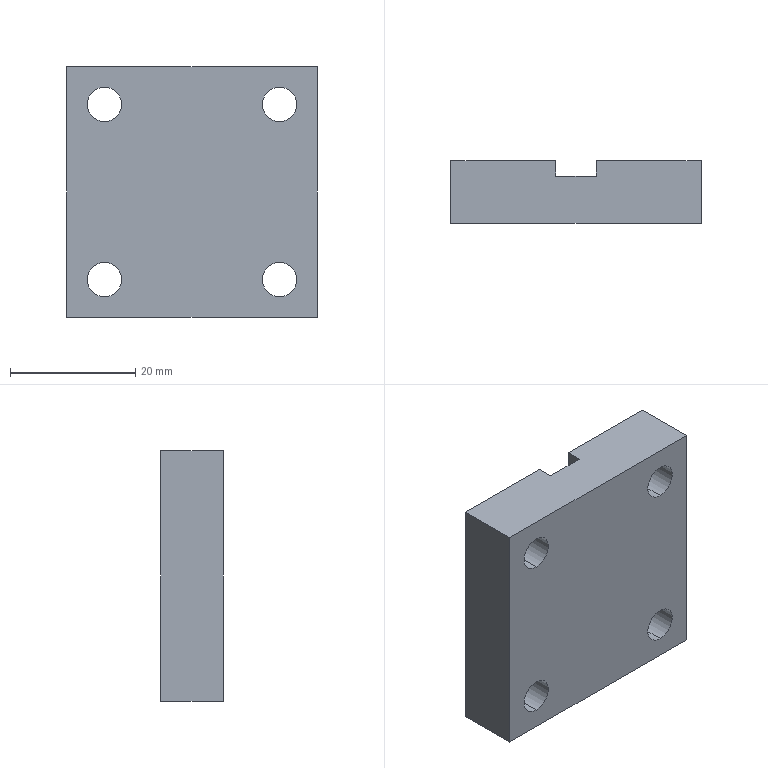Part | STEP file | magnetizing cover plate | 1 solid | 18 faces | box 40 x 10 x 40 mm | volume 14400 mm3 | plane 10 | cylinder 8 | commonest cylinder face diameters 5.5 x8
STEP:
#1=CARTESIAN_POINT('',(0.,0.,0.));
#2=DIRECTION('',(0.,0.,1.));
#3=DIRECTION('',(1.,0.,0.));
#4=AXIS2_PLACEMENT_3D('',#1,#2,#3);
#5=CARTESIAN_POINT('',(14.,5.,31.25));
#6=VERTEX_POINT('',#5);
#7=CARTESIAN_POINT('',(14.,-5.,31.25));
#8=VERTEX_POINT('',#7);
#9=CARTESIAN_POINT('',(14.,35.,31.25));
#10=DIRECTION('',(0.,-1.,0.));
#11=VECTOR('',#10,1.);
#12=LINE('',#9,#11);
#13=CARTESIAN_POINT('',(14.,35.,34.));
#14=DIRECTION('',(0.,-1.,0.));
#15=DIRECTION('',(0.,0.,-1.));
#16=AXIS2_PLACEMENT_3D('',#13,#14,#15);
#17=CYLINDRICAL_SURFACE('',#16,2.75);
#18=CARTESIAN_POINT('',(6.283,0.));
#19=DIRECTION('',(0.,1.));
#20=VECTOR('',#19,1.);
#21=LINE('',#18,#20);
#22=(GEOMETRIC_REPRESENTATION_CONTEXT(2)PARAMETRIC_REPRESENTATION_CONTEXT()REPRESENTATION_CONTEXT('',''));
#23=DEFINITIONAL_REPRESENTATION('',(#21),#22);
#24=PCURVE('',#17,#23);
#25=CARTESIAN_POINT('',(14.,35.,34.));
#26=DIRECTION('',(0.,-1.,0.));
#27=DIRECTION('',(0.,0.,-1.));
#28=AXIS2_PLACEMENT_3D('',#25,#26,#27);
#29=CYLINDRICAL_SURFACE('',#28,2.75);
#30=CARTESIAN_POINT('',(0.,0.));
#31=DIRECTION('',(0.,1.));
#32=VECTOR('',#31,1.);
#33=LINE('',#30,#32);
#34=(GEOMETRIC_REPRESENTATION_CONTEXT(2)PARAMETRIC_REPRESENTATION_CONTEXT()REPRESENTATION_CONTEXT('',''));
#35=DEFINITIONAL_REPRESENTATION('',(#33),#34);
#36=PCURVE('',#29,#35);
#37=SURFACE_CURVE('',#12,(#24,#36),.PCURVE_S1.);
#38=EDGE_CURVE('',#6,#8,#37,.T.);
#39=ORIENTED_EDGE('',*,*,#38,.T.);
#40=CARTESIAN_POINT('',(14.,-5.,36.75));
#41=VERTEX_POINT('',#40);
#42=CARTESIAN_POINT('',(14.,-5.,34.));
#43=DIRECTION('',(0.,-1.,0.));
#44=DIRECTION('',(0.,0.,-1.));
#45=AXIS2_PLACEMENT_3D('',#42,#43,#44);
#46=CIRCLE('',#45,2.75);
#47=CARTESIAN_POINT('',(0.,40.));
#48=DIRECTION('',(1.,0.));
#49=VECTOR('',#48,1.);
#50=LINE('',#47,#49);
#51=(GEOMETRIC_REPRESENTATION_CONTEXT(2)PARAMETRIC_REPRESENTATION_CONTEXT()REPRESENTATION_CONTEXT('',''));
#52=DEFINITIONAL_REPRESENTATION('',(#50),#51);
#53=PCURVE('',#17,#52);
#54=CARTESIAN_POINT('',(-20.,-5.,40.));
#55=DIRECTION('',(0.,1.,0.));
#56=DIRECTION('',(0.,0.,1.));
#57=AXIS2_PLACEMENT_3D('',#54,#55,#56);
#58=PLANE('',#57);
#59=CARTESIAN_POINT('',(-8.75,34.));
#60=CARTESIAN_POINT('',(-8.75,38.763));
#61=CARTESIAN_POINT('',(-4.625,36.382));
#62=CARTESIAN_POINT('',(-0.5,34.));
#63=CARTESIAN_POINT('',(-4.625,31.618));
#64=CARTESIAN_POINT('',(-8.75,29.237));
#65=CARTESIAN_POINT('',(-8.75,34.));
#66=(BOUNDED_CURVE()B_SPLINE_CURVE(2,(#59,#60,#61,#62,#63,#64,#65),.UNSPECIFIED.,.T.,.F.)B_SPLINE_CURVE_WITH_KNOTS((1,2,2,2,2,1),(-2.094,0.,2.094,4.189,6.283,8.378),.UNSPECIFIED.)CURVE()GEOMETRIC_REPRESENTATION_ITEM()RATIONAL_B_SPLINE_CURVE((1.,0.5,1.,0.5,1.,0.5,1.))REPRESENTATION_ITEM(''));
#67=(GEOMETRIC_REPRESENTATION_CONTEXT(2)PARAMETRIC_REPRESENTATION_CONTEXT()REPRESENTATION_CONTEXT('',''));
#68=DEFINITIONAL_REPRESENTATION('',(#66),#67);
#69=PCURVE('',#58,#68);
#70=SURFACE_CURVE('',#46,(#53,#69),.PCURVE_S1.);
#71=EDGE_CURVE('',#41,#8,#70,.T.);
#72=ORIENTED_EDGE('',*,*,#71,.F.);
#73=CARTESIAN_POINT('',(14.,5.,36.75));
#74=VERTEX_POINT('',#73);
#75=CARTESIAN_POINT('',(14.,35.,36.75));
#76=DIRECTION('',(0.,-1.,0.));
#77=VECTOR('',#76,1.);
#78=LINE('',#75,#77);
#79=CARTESIAN_POINT('',(3.142,0.));
#80=DIRECTION('',(0.,1.));
#81=VECTOR('',#80,1.);
#82=LINE('',#79,#81);
#83=(GEOMETRIC_REPRESENTATION_CONTEXT(2)PARAMETRIC_REPRESENTATION_CONTEXT()REPRESENTATION_CONTEXT('',''));
#84=DEFINITIONAL_REPRESENTATION('',(#82),#83);
#85=PCURVE('',#17,#84);
#86=CARTESIAN_POINT('',(3.142,0.));
#87=DIRECTION('',(0.,1.));
#88=VECTOR('',#87,1.);
#89=LINE('',#86,#88);
#90=(GEOMETRIC_REPRESENTATION_CONTEXT(2)PARAMETRIC_REPRESENTATION_CONTEXT()REPRESENTATION_CONTEXT('',''));
#91=DEFINITIONAL_REPRESENTATION('',(#89),#90);
#92=PCURVE('',#29,#91);
#93=SURFACE_CURVE('',#78,(#85,#92),.PCURVE_S1.);
#94=EDGE_CURVE('',#74,#41,#93,.T.);
#95=ORIENTED_EDGE('',*,*,#94,.F.);
#96=CARTESIAN_POINT('',(14.,5.,34.));
#97=DIRECTION('',(0.,-1.,0.));
#98=DIRECTION('',(1.,0.,0.));
#99=AXIS2_PLACEMENT_3D('',#96,#97,#98);
#100=CIRCLE('',#99,2.75);
#101=CARTESIAN_POINT('',(1.571,30.));
#102=DIRECTION('',(1.,0.));
#103=VECTOR('',#102,1.);
#104=LINE('',#101,#103);
#105=(GEOMETRIC_REPRESENTATION_CONTEXT(2)PARAMETRIC_REPRESENTATION_CONTEXT()REPRESENTATION_CONTEXT('',''));
#106=DEFINITIONAL_REPRESENTATION('',(#104),#105);
#107=PCURVE('',#17,#106);
#108=CARTESIAN_POINT('',(3.25,5.,40.));
#109=DIRECTION('',(0.,-1.,0.));
#110=DIRECTION('',(1.,0.,0.));
#111=AXIS2_PLACEMENT_3D('',#108,#109,#110);
#112=PLANE('',#111);
#113=CARTESIAN_POINT('',(10.75,-6.));
#114=DIRECTION('',(1.,0.));
#115=AXIS2_PLACEMENT_2D('',#113,#114);
#116=CIRCLE('',#115,2.75);
#117=(GEOMETRIC_REPRESENTATION_CONTEXT(2)PARAMETRIC_REPRESENTATION_CONTEXT()REPRESENTATION_CONTEXT('',''));
#118=DEFINITIONAL_REPRESENTATION('',(#116),#117);
#119=PCURVE('',#112,#118);
#120=SURFACE_CURVE('',#100,(#107,#119),.PCURVE_S1.);
#121=EDGE_CURVE('',#74,#6,#120,.T.);
#122=ORIENTED_EDGE('',*,*,#121,.T.);
#123=EDGE_LOOP('',(#39,#72,#95,#122));
#124=FACE_BOUND('',#123,.F.);
#125=ADVANCED_FACE('',(#124),#17,.F.);
#126=CARTESIAN_POINT('',(14.,5.,3.25));
#127=VERTEX_POINT('',#126);
#128=CARTESIAN_POINT('',(14.,-5.,3.25));
#129=VERTEX_POINT('',#128);
#130=CARTESIAN_POINT('',(14.,35.,3.25));
#131=DIRECTION('',(0.,-1.,0.));
#132=VECTOR('',#131,1.);
#133=LINE('',#130,#132);
#134=CARTESIAN_POINT('',(14.,35.,6.));
#135=DIRECTION('',(0.,-1.,0.));
#136=DIRECTION('',(0.,0.,-1.));
#137=AXIS2_PLACEMENT_3D('',#134,#135,#136);
#138=CYLINDRICAL_SURFACE('',#137,2.75);
#139=CARTESIAN_POINT('',(6.283,0.));
#140=DIRECTION('',(0.,1.));
#141=VECTOR('',#140,1.);
#142=LINE('',#139,#141);
#143=(GEOMETRIC_REPRESENTATION_CONTEXT(2)PARAMETRIC_REPRESENTATION_CONTEXT()REPRESENTATION_CONTEXT('',''));
#144=DEFINITIONAL_REPRESENTATION('',(#142),#143);
#145=PCURVE('',#138,#144);
#146=CARTESIAN_POINT('',(14.,35.,6.));
#147=DIRECTION('',(0.,-1.,0.));
#148=DIRECTION('',(0.,0.,-1.));
#149=AXIS2_PLACEMENT_3D('',#146,#147,#148);
#150=CYLINDRICAL_SURFACE('',#149,2.75);
#151=CARTESIAN_POINT('',(0.,0.));
#152=DIRECTION('',(0.,1.));
#153=VECTOR('',#152,1.);
#154=LINE('',#151,#153);
#155=(GEOMETRIC_REPRESENTATION_CONTEXT(2)PARAMETRIC_REPRESENTATION_CONTEXT()REPRESENTATION_CONTEXT('',''));
#156=DEFINITIONAL_REPRESENTATION('',(#154),#155);
#157=PCURVE('',#150,#156);
#158=SURFACE_CURVE('',#133,(#145,#157),.PCURVE_S1.);
#159=EDGE_CURVE('',#127,#129,#158,.T.);
#160=ORIENTED_EDGE('',*,*,#159,.T.);
#161=CARTESIAN_POINT('',(14.,-5.,8.75));
#162=VERTEX_POINT('',#161);
#163=CARTESIAN_POINT('',(14.,-5.,6.));
#164=DIRECTION('',(0.,-1.,0.));
#165=DIRECTION('',(0.,0.,-1.));
#166=AXIS2_PLACEMENT_3D('',#163,#164,#165);
#167=CIRCLE('',#166,2.75);
#168=CARTESIAN_POINT('',(0.,40.));
#169=DIRECTION('',(1.,0.));
#170=VECTOR('',#169,1.);
#171=LINE('',#168,#170);
#172=(GEOMETRIC_REPRESENTATION_CONTEXT(2)PARAMETRIC_REPRESENTATION_CONTEXT()REPRESENTATION_CONTEXT('',''));
#173=DEFINITIONAL_REPRESENTATION('',(#171),#172);
#174=PCURVE('',#138,#173);
#175=CARTESIAN_POINT('',(-36.75,34.));
#176=CARTESIAN_POINT('',(-36.75,38.763));
#177=CARTESIAN_POINT('',(-32.625,36.382));
#178=CARTESIAN_POINT('',(-28.5,34.));
#179=CARTESIAN_POINT('',(-32.625,31.618));
#180=CARTESIAN_POINT('',(-36.75,29.237));
#181=CARTESIAN_POINT('',(-36.75,34.));
#182=(BOUNDED_CURVE()B_SPLINE_CURVE(2,(#175,#176,#177,#178,#179,#180,#181),.UNSPECIFIED.,.T.,.F.)B_SPLINE_CURVE_WITH_KNOTS((1,2,2,2,2,1),(-2.094,0.,2.094,4.189,6.283,8.378),.UNSPECIFIED.)CURVE()GEOMETRIC_REPRESENTATION_ITEM()RATIONAL_B_SPLINE_CURVE((1.,0.5,1.,0.5,1.,0.5,1.))REPRESENTATION_ITEM(''));
#183=(GEOMETRIC_REPRESENTATION_CONTEXT(2)PARAMETRIC_REPRESENTATION_CONTEXT()REPRESENTATION_CONTEXT('',''));
#184=DEFINITIONAL_REPRESENTATION('',(#182),#183);
#185=PCURVE('',#58,#184);
#186=SURFACE_CURVE('',#167,(#174,#185),.PCURVE_S1.);
#187=EDGE_CURVE('',#162,#129,#186,.T.);
#188=ORIENTED_EDGE('',*,*,#187,.F.);
#189=CARTESIAN_POINT('',(14.,5.,8.75));
#190=VERTEX_POINT('',#189);
#191=CARTESIAN_POINT('',(14.,35.,8.75));
#192=DIRECTION('',(0.,-1.,0.));
#193=VECTOR('',#192,1.);
#194=LINE('',#191,#193);
#195=CARTESIAN_POINT('',(3.142,0.));
#196=DIRECTION('',(0.,1.));
#197=VECTOR('',#196,1.);
#198=LINE('',#195,#197);
#199=(GEOMETRIC_REPRESENTATION_CONTEXT(2)PARAMETRIC_REPRESENTATION_CONTEXT()REPRESENTATION_CONTEXT('',''));
#200=DEFINITIONAL_REPRESENTATION('',(#198),#199);
#201=PCURVE('',#138,#200);
#202=CARTESIAN_POINT('',(3.142,0.));
#203=DIRECTION('',(0.,1.));
#204=VECTOR('',#203,1.);
#205=LINE('',#202,#204);
#206=(GEOMETRIC_REPRESENTATION_CONTEXT(2)PARAMETRIC_REPRESENTATION_CONTEXT()REPRESENTATION_CONTEXT('',''));
#207=DEFINITIONAL_REPRESENTATION('',(#205),#206);
#208=PCURVE('',#150,#207);
#209=SURFACE_CURVE('',#194,(#201,#208),.PCURVE_S1.);
#210=EDGE_CURVE('',#190,#162,#209,.T.);
#211=ORIENTED_EDGE('',*,*,#210,.F.);
#212=CARTESIAN_POINT('',(14.,5.,6.));
#213=DIRECTION('',(0.,-1.,0.));
#214=DIRECTION('',(1.,0.,0.));
#215=AXIS2_PLACEMENT_3D('',#212,#213,#214);
#216=CIRCLE('',#215,2.75);
#217=CARTESIAN_POINT('',(1.571,30.));
#218=DIRECTION('',(1.,0.));
#219=VECTOR('',#218,1.);
#220=LINE('',#217,#219);
#221=(GEOMETRIC_REPRESENTATION_CONTEXT(2)PARAMETRIC_REPRESENTATION_CONTEXT()REPRESENTATION_CONTEXT('',''));
#222=DEFINITIONAL_REPRESENTATION('',(#220),#221);
#223=PCURVE('',#138,#222);
#224=CARTESIAN_POINT('',(10.75,-34.));
#225=DIRECTION('',(1.,0.));
#226=AXIS2_PLACEMENT_2D('',#224,#225);
#227=CIRCLE('',#226,2.75);
#228=(GEOMETRIC_REPRESENTATION_CONTEXT(2)PARAMETRIC_REPRESENTATION_CONTEXT()REPRESENTATION_CONTEXT('',''));
#229=DEFINITIONAL_REPRESENTATION('',(#227),#228);
#230=PCURVE('',#112,#229);
#231=SURFACE_CURVE('',#216,(#223,#230),.PCURVE_S1.);
#232=EDGE_CURVE('',#190,#127,#231,.T.);
#233=ORIENTED_EDGE('',*,*,#232,.T.);
#234=EDGE_LOOP('',(#160,#188,#211,#233));
#235=FACE_BOUND('',#234,.F.);
#236=ADVANCED_FACE('',(#235),#138,.F.);
#237=CARTESIAN_POINT('',(-14.,5.,3.25));
#238=VERTEX_POINT('',#237);
#239=CARTESIAN_POINT('',(-14.,-5.,3.25));
#240=VERTEX_POINT('',#239);
#241=CARTESIAN_POINT('',(-14.,35.,3.25));
#242=DIRECTION('',(0.,-1.,0.));
#243=VECTOR('',#242,1.);
#244=LINE('',#241,#243);
#245=CARTESIAN_POINT('',(-14.,35.,6.));
#246=DIRECTION('',(0.,-1.,0.));
#247=DIRECTION('',(0.,0.,-1.));
#248=AXIS2_PLACEMENT_3D('',#245,#246,#247);
#249=CYLINDRICAL_SURFACE('',#248,2.75);
#250=CARTESIAN_POINT('',(6.283,0.));
#251=DIRECTION('',(0.,1.));
#252=VECTOR('',#251,1.);
#253=LINE('',#250,#252);
#254=(GEOMETRIC_REPRESENTATION_CONTEXT(2)PARAMETRIC_REPRESENTATION_CONTEXT()REPRESENTATION_CONTEXT('',''));
#255=DEFINITIONAL_REPRESENTATION('',(#253),#254);
#256=PCURVE('',#249,#255);
#257=CARTESIAN_POINT('',(-14.,35.,6.));
#258=DIRECTION('',(0.,-1.,0.));
#259=DIRECTION('',(0.,0.,-1.));
#260=AXIS2_PLACEMENT_3D('',#257,#258,#259);
#261=CYLINDRICAL_SURFACE('',#260,2.75);
#262=CARTESIAN_POINT('',(0.,0.));
#263=DIRECTION('',(0.,1.));
#264=VECTOR('',#263,1.);
#265=LINE('',#262,#264);
#266=(GEOMETRIC_REPRESENTATION_CONTEXT(2)PARAMETRIC_REPRESENTATION_CONTEXT()REPRESENTATION_CONTEXT('',''));
#267=DEFINITIONAL_REPRESENTATION('',(#265),#266);
#268=PCURVE('',#261,#267);
#269=SURFACE_CURVE('',#244,(#256,#268),.PCURVE_S1.);
#270=EDGE_CURVE('',#238,#240,#269,.T.);
#271=ORIENTED_EDGE('',*,*,#270,.T.);
#272=CARTESIAN_POINT('',(-14.,-5.,8.75));
#273=VERTEX_POINT('',#272);
#274=CARTESIAN_POINT('',(-14.,-5.,6.));
#275=DIRECTION('',(0.,-1.,0.));
#276=DIRECTION('',(0.,0.,-1.));
#277=AXIS2_PLACEMENT_3D('',#274,#275,#276);
#278=CIRCLE('',#277,2.75);
#279=CARTESIAN_POINT('',(0.,40.));
#280=DIRECTION('',(1.,0.));
#281=VECTOR('',#280,1.);
#282=LINE('',#279,#281);
#283=(GEOMETRIC_REPRESENTATION_CONTEXT(2)PARAMETRIC_REPRESENTATION_CONTEXT()REPRESENTATION_CONTEXT('',''));
#284=DEFINITIONAL_REPRESENTATION('',(#282),#283);
#285=PCURVE('',#249,#284);
#286=CARTESIAN_POINT('',(-36.75,6.));
#287=CARTESIAN_POINT('',(-36.75,10.763));
#288=CARTESIAN_POINT('',(-32.625,8.382));
#289=CARTESIAN_POINT('',(-28.5,6.));
#290=CARTESIAN_POINT('',(-32.625,3.618));
#291=CARTESIAN_POINT('',(-36.75,1.237));
#292=CARTESIAN_POINT('',(-36.75,6.));
#293=(BOUNDED_CURVE()B_SPLINE_CURVE(2,(#286,#287,#288,#289,#290,#291,#292),.UNSPECIFIED.,.T.,.F.)B_SPLINE_CURVE_WITH_KNOTS((1,2,2,2,2,1),(-2.094,0.,2.094,4.189,6.283,8.378),.UNSPECIFIED.)CURVE()GEOMETRIC_REPRESENTATION_ITEM()RATIONAL_B_SPLINE_CURVE((1.,0.5,1.,0.5,1.,0.5,1.))REPRESENTATION_ITEM(''));
#294=(GEOMETRIC_REPRESENTATION_CONTEXT(2)PARAMETRIC_REPRESENTATION_CONTEXT()REPRESENTATION_CONTEXT('',''));
#295=DEFINITIONAL_REPRESENTATION('',(#293),#294);
#296=PCURVE('',#58,#295);
#297=SURFACE_CURVE('',#278,(#285,#296),.PCURVE_S1.);
#298=EDGE_CURVE('',#273,#240,#297,.T.);
#299=ORIENTED_EDGE('',*,*,#298,.F.);
#300=CARTESIAN_POINT('',(-14.,5.,8.75));
#301=VERTEX_POINT('',#300);
#302=CARTESIAN_POINT('',(-14.,35.,8.75));
#303=DIRECTION('',(0.,-1.,0.));
#304=VECTOR('',#303,1.);
#305=LINE('',#302,#304);
#306=CARTESIAN_POINT('',(3.142,0.));
#307=DIRECTION('',(0.,1.));
#308=VECTOR('',#307,1.);
#309=LINE('',#306,#308);
#310=(GEOMETRIC_REPRESENTATION_CONTEXT(2)PARAMETRIC_REPRESENTATION_CONTEXT()REPRESENTATION_CONTEXT('',''));
#311=DEFINITIONAL_REPRESENTATION('',(#309),#310);
#312=PCURVE('',#249,#311);
#313=CARTESIAN_POINT('',(3.142,0.));
#314=DIRECTION('',(0.,1.));
#315=VECTOR('',#314,1.);
#316=LINE('',#313,#315);
#317=(GEOMETRIC_REPRESENTATION_CONTEXT(2)PARAMETRIC_REPRESENTATION_CONTEXT()REPRESENTATION_CONTEXT('',''));
#318=DEFINITIONAL_REPRESENTATION('',(#316),#317);
#319=PCURVE('',#261,#318);
#320=SURFACE_CURVE('',#305,(#312,#319),.PCURVE_S1.);
#321=EDGE_CURVE('',#301,#273,#320,.T.);
#322=ORIENTED_EDGE('',*,*,#321,.F.);
#323=CARTESIAN_POINT('',(-14.,5.,6.));
#324=DIRECTION('',(0.,-1.,0.));
#325=DIRECTION('',(0.,0.,-1.));
#326=AXIS2_PLACEMENT_3D('',#323,#324,#325);
#327=CIRCLE('',#326,2.75);
#328=CARTESIAN_POINT('',(0.,30.));
#329=DIRECTION('',(1.,0.));
#330=VECTOR('',#329,1.);
#331=LINE('',#328,#330);
#332=(GEOMETRIC_REPRESENTATION_CONTEXT(2)PARAMETRIC_REPRESENTATION_CONTEXT()REPRESENTATION_CONTEXT('',''));
#333=DEFINITIONAL_REPRESENTATION('',(#331),#332);
#334=PCURVE('',#249,#333);
#335=CARTESIAN_POINT('',(-20.,5.,40.));
#336=DIRECTION('',(0.,-1.,0.));
#337=DIRECTION('',(0.,0.,-1.));
#338=AXIS2_PLACEMENT_3D('',#335,#336,#337);
#339=PLANE('',#338);
#340=CARTESIAN_POINT('',(34.,6.));
#341=DIRECTION('',(1.,0.));
#342=AXIS2_PLACEMENT_2D('',#340,#341);
#343=CIRCLE('',#342,2.75);
#344=(GEOMETRIC_REPRESENTATION_CONTEXT(2)PARAMETRIC_REPRESENTATION_CONTEXT()REPRESENTATION_CONTEXT('',''));
#345=DEFINITIONAL_REPRESENTATION('',(#343),#344);
#346=PCURVE('',#339,#345);
#347=SURFACE_CURVE('',#327,(#334,#346),.PCURVE_S1.);
#348=EDGE_CURVE('',#301,#238,#347,.T.);
#349=ORIENTED_EDGE('',*,*,#348,.T.);
#350=EDGE_LOOP('',(#271,#299,#322,#349));
#351=FACE_BOUND('',#350,.F.);
#352=ADVANCED_FACE('',(#351),#249,.F.);
#353=CARTESIAN_POINT('',(-14.,5.,31.25));
#354=VERTEX_POINT('',#353);
#355=CARTESIAN_POINT('',(-14.,-5.,31.25));
#356=VERTEX_POINT('',#355);
#357=CARTESIAN_POINT('',(-14.,35.,31.25));
#358=DIRECTION('',(0.,-1.,0.));
#359=VECTOR('',#358,1.);
#360=LINE('',#357,#359);
#361=CARTESIAN_POINT('',(-14.,35.,34.));
#362=DIRECTION('',(0.,-1.,0.));
#363=DIRECTION('',(0.,0.,-1.));
#364=AXIS2_PLACEMENT_3D('',#361,#362,#363);
#365=CYLINDRICAL_SURFACE('',#364,2.75);
#366=CARTESIAN_POINT('',(6.283,0.));
#367=DIRECTION('',(0.,1.));
#368=VECTOR('',#367,1.);
#369=LINE('',#366,#368);
#370=(GEOMETRIC_REPRESENTATION_CONTEXT(2)PARAMETRIC_REPRESENTATION_CONTEXT()REPRESENTATION_CONTEXT('',''));
#371=DEFINITIONAL_REPRESENTATION('',(#369),#370);
#372=PCURVE('',#365,#371);
#373=CARTESIAN_POINT('',(-14.,35.,34.));
#374=DIRECTION('',(0.,-1.,0.));
#375=DIRECTION('',(0.,0.,-1.));
#376=AXIS2_PLACEMENT_3D('',#373,#374,#375);
#377=CYLINDRICAL_SURFACE('',#376,2.75);
#378=CARTESIAN_POINT('',(0.,0.));
#379=DIRECTION('',(0.,1.));
#380=VECTOR('',#379,1.);
#381=LINE('',#378,#380);
#382=(GEOMETRIC_REPRESENTATION_CONTEXT(2)PARAMETRIC_REPRESENTATION_CONTEXT()REPRESENTATION_CONTEXT('',''));
#383=DEFINITIONAL_REPRESENTATION('',(#381),#382);
#384=PCURVE('',#377,#383);
#385=SURFACE_CURVE('',#360,(#372,#384),.PCURVE_S1.);
#386=EDGE_CURVE('',#354,#356,#385,.T.);
#387=ORIENTED_EDGE('',*,*,#386,.T.);
#388=CARTESIAN_POINT('',(-14.,-5.,36.75));
#389=VERTEX_POINT('',#388);
#390=CARTESIAN_POINT('',(-14.,-5.,34.));
#391=DIRECTION('',(0.,-1.,0.));
#392=DIRECTION('',(0.,0.,-1.));
#393=AXIS2_PLACEMENT_3D('',#390,#391,#392);
#394=CIRCLE('',#393,2.75);
#395=CARTESIAN_POINT('',(0.,40.));
#396=DIRECTION('',(1.,0.));
#397=VECTOR('',#396,1.);
#398=LINE('',#395,#397);
#399=(GEOMETRIC_REPRESENTATION_CONTEXT(2)PARAMETRIC_REPRESENTATION_CONTEXT()REPRESENTATION_CONTEXT('',''));
#400=DEFINITIONAL_REPRESENTATION('',(#398),#399);
#401=PCURVE('',#365,#400);
#402=CARTESIAN_POINT('',(-8.75,6.));
#403=CARTESIAN_POINT('',(-8.75,10.763));
#404=CARTESIAN_POINT('',(-4.625,8.382));
#405=CARTESIAN_POINT('',(-0.5,6.));
#406=CARTESIAN_POINT('',(-4.625,3.618));
#407=CARTESIAN_POINT('',(-8.75,1.237));
#408=CARTESIAN_POINT('',(-8.75,6.));
#409=(BOUNDED_CURVE()B_SPLINE_CURVE(2,(#402,#403,#404,#405,#406,#407,#408),.UNSPECIFIED.,.T.,.F.)B_SPLINE_CURVE_WITH_KNOTS((1,2,2,2,2,1),(-2.094,0.,2.094,4.189,6.283,8.378),.UNSPECIFIED.)CURVE()GEOMETRIC_REPRESENTATION_ITEM()RATIONAL_B_SPLINE_CURVE((1.,0.5,1.,0.5,1.,0.5,1.))REPRESENTATION_ITEM(''));
#410=(GEOMETRIC_REPRESENTATION_CONTEXT(2)PARAMETRIC_REPRESENTATION_CONTEXT()REPRESENTATION_CONTEXT('',''));
#411=DEFINITIONAL_REPRESENTATION('',(#409),#410);
#412=PCURVE('',#58,#411);
#413=SURFACE_CURVE('',#394,(#401,#412),.PCURVE_S1.);
#414=EDGE_CURVE('',#389,#356,#413,.T.);
#415=ORIENTED_EDGE('',*,*,#414,.F.);
#416=CARTESIAN_POINT('',(-14.,5.,36.75));
#417=VERTEX_POINT('',#416);
#418=CARTESIAN_POINT('',(-14.,35.,36.75));
#419=DIRECTION('',(0.,-1.,0.));
#420=VECTOR('',#419,1.);
#421=LINE('',#418,#420);
#422=CARTESIAN_POINT('',(3.142,0.));
#423=DIRECTION('',(0.,1.));
#424=VECTOR('',#423,1.);
#425=LINE('',#422,#424);
#426=(GEOMETRIC_REPRESENTATION_CONTEXT(2)PARAMETRIC_REPRESENTATION_CONTEXT()REPRESENTATION_CONTEXT('',''));
#427=DEFINITIONAL_REPRESENTATION('',(#425),#426);
#428=PCURVE('',#365,#427);
#429=CARTESIAN_POINT('',(3.142,0.));
#430=DIRECTION('',(0.,1.));
#431=VECTOR('',#430,1.);
#432=LINE('',#429,#431);
#433=(GEOMETRIC_REPRESENTATION_CONTEXT(2)PARAMETRIC_REPRESENTATION_CONTEXT()REPRESENTATION_CONTEXT('',''));
#434=DEFINITIONAL_REPRESENTATION('',(#432),#433);
#435=PCURVE('',#377,#434);
#436=SURFACE_CURVE('',#421,(#428,#435),.PCURVE_S1.);
#437=EDGE_CURVE('',#417,#389,#436,.T.);
#438=ORIENTED_EDGE('',*,*,#437,.F.);
#439=CARTESIAN_POINT('',(-14.,5.,34.));
#440=DIRECTION('',(0.,-1.,0.));
#441=DIRECTION('',(0.,0.,-1.));
#442=AXIS2_PLACEMENT_3D('',#439,#440,#441);
#443=CIRCLE('',#442,2.75);
#444=CARTESIAN_POINT('',(0.,30.));
#445=DIRECTION('',(1.,0.));
#446=VECTOR('',#445,1.);
#447=LINE('',#444,#446);
#448=(GEOMETRIC_REPRESENTATION_CONTEXT(2)PARAMETRIC_REPRESENTATION_CONTEXT()REPRESENTATION_CONTEXT('',''));
#449=DEFINITIONAL_REPRESENTATION('',(#447),#448);
#450=PCURVE('',#365,#449);
#451=CARTESIAN_POINT('',(6.,6.));
#452=DIRECTION('',(1.,0.));
#453=AXIS2_PLACEMENT_2D('',#451,#452);
#454=CIRCLE('',#453,2.75);
#455=(GEOMETRIC_REPRESENTATION_CONTEXT(2)PARAMETRIC_REPRESENTATION_CONTEXT()REPRESENTATION_CONTEXT('',''));
#456=DEFINITIONAL_REPRESENTATION('',(#454),#455);
#457=PCURVE('',#339,#456);
#458=SURFACE_CURVE('',#443,(#450,#457),.PCURVE_S1.);
#459=EDGE_CURVE('',#417,#354,#458,.T.);
#460=ORIENTED_EDGE('',*,*,#459,.T.);
#461=EDGE_LOOP('',(#387,#415,#438,#460));
#462=FACE_BOUND('',#461,.F.);
#463=ADVANCED_FACE('',(#462),#365,.F.);
#464=CARTESIAN_POINT('',(20.,-5.,0.));
#465=VERTEX_POINT('',#464);
#466=CARTESIAN_POINT('',(20.,5.,0.));
#467=VERTEX_POINT('',#466);
#468=CARTESIAN_POINT('',(20.,5.,0.));
#469=DIRECTION('',(0.,1.,0.));
#470=VECTOR('',#469,1.);
#471=LINE('',#468,#470);
#472=CARTESIAN_POINT('',(20.,5.,40.));
#473=DIRECTION('',(-1.,0.,0.));
#474=DIRECTION('',(0.,0.,1.));
#475=AXIS2_PLACEMENT_3D('',#472,#473,#474);
#476=PLANE('',#475);
#477=CARTESIAN_POINT('',(-40.,0.));
#478=DIRECTION('',(0.,1.));
#479=VECTOR('',#478,1.);
#480=LINE('',#477,#479);
#481=(GEOMETRIC_REPRESENTATION_CONTEXT(2)PARAMETRIC_REPRESENTATION_CONTEXT()REPRESENTATION_CONTEXT('',''));
#482=DEFINITIONAL_REPRESENTATION('',(#480),#481);
#483=PCURVE('',#476,#482);
#484=CARTESIAN_POINT('',(20.,-5.,0.));
#485=DIRECTION('',(0.,0.,1.));
#486=DIRECTION('',(1.,0.,0.));
#487=AXIS2_PLACEMENT_3D('',#484,#485,#486);
#488=PLANE('',#487);
#489=CARTESIAN_POINT('',(0.,10.));
#490=DIRECTION('',(0.,1.));
#491=VECTOR('',#490,1.);
#492=LINE('',#489,#491);
#493=(GEOMETRIC_REPRESENTATION_CONTEXT(2)PARAMETRIC_REPRESENTATION_CONTEXT()REPRESENTATION_CONTEXT('',''));
#494=DEFINITIONAL_REPRESENTATION('',(#492),#493);
#495=PCURVE('',#488,#494);
#496=SURFACE_CURVE('',#471,(#483,#495),.PCURVE_S1.);
#497=EDGE_CURVE('',#465,#467,#496,.T.);
#498=ORIENTED_EDGE('',*,*,#497,.T.);
#499=CARTESIAN_POINT('',(20.,5.,40.));
#500=VERTEX_POINT('',#499);
#501=CARTESIAN_POINT('',(20.,5.,40.));
#502=DIRECTION('',(0.,0.,-1.));
#503=VECTOR('',#502,1.);
#504=LINE('',#501,#503);
#505=CARTESIAN_POINT('',(0.,0.));
#506=DIRECTION('',(-1.,0.));
#507=VECTOR('',#506,1.);
#508=LINE('',#505,#507);
#509=(GEOMETRIC_REPRESENTATION_CONTEXT(2)PARAMETRIC_REPRESENTATION_CONTEXT()REPRESENTATION_CONTEXT('',''));
#510=DEFINITIONAL_REPRESENTATION('',(#508),#509);
#511=PCURVE('',#476,#510);
#512=CARTESIAN_POINT('',(16.75,0.));
#513=DIRECTION('',(0.,-1.));
#514=VECTOR('',#513,1.);
#515=LINE('',#512,#514);
#516=(GEOMETRIC_REPRESENTATION_CONTEXT(2)PARAMETRIC_REPRESENTATION_CONTEXT()REPRESENTATION_CONTEXT('',''));
#517=DEFINITIONAL_REPRESENTATION('',(#515),#516);
#518=PCURVE('',#112,#517);
#519=SURFACE_CURVE('',#504,(#511,#518),.PCURVE_S1.);
#520=EDGE_CURVE('',#500,#467,#519,.T.);
#521=ORIENTED_EDGE('',*,*,#520,.F.);
#522=CARTESIAN_POINT('',(20.,-5.,40.));
#523=VERTEX_POINT('',#522);
#524=CARTESIAN_POINT('',(20.,5.,40.));
#525=DIRECTION('',(0.,1.,0.));
#526=VECTOR('',#525,1.);
#527=LINE('',#524,#526);
#528=CARTESIAN_POINT('',(0.,0.));
#529=DIRECTION('',(0.,1.));
#530=VECTOR('',#529,1.);
#531=LINE('',#528,#530);
#532=(GEOMETRIC_REPRESENTATION_CONTEXT(2)PARAMETRIC_REPRESENTATION_CONTEXT()REPRESENTATION_CONTEXT('',''));
#533=DEFINITIONAL_REPRESENTATION('',(#531),#532);
#534=PCURVE('',#476,#533);
#535=CARTESIAN_POINT('',(20.,-5.,40.));
#536=DIRECTION('',(0.,0.,1.));
#537=DIRECTION('',(1.,0.,0.));
#538=AXIS2_PLACEMENT_3D('',#535,#536,#537);
#539=PLANE('',#538);
#540=CARTESIAN_POINT('',(0.,10.));
#541=DIRECTION('',(0.,1.));
#542=VECTOR('',#541,1.);
#543=LINE('',#540,#542);
#544=(GEOMETRIC_REPRESENTATION_CONTEXT(2)PARAMETRIC_REPRESENTATION_CONTEXT()REPRESENTATION_CONTEXT('',''));
#545=DEFINITIONAL_REPRESENTATION('',(#543),#544);
#546=PCURVE('',#539,#545);
#547=SURFACE_CURVE('',#527,(#534,#546),.PCURVE_S1.);
#548=EDGE_CURVE('',#523,#500,#547,.T.);
#549=ORIENTED_EDGE('',*,*,#548,.F.);
#550=CARTESIAN_POINT('',(20.,-5.,40.));
#551=DIRECTION('',(0.,0.,-1.));
#552=VECTOR('',#551,1.);
#553=LINE('',#550,#552);
#554=CARTESIAN_POINT('',(0.,-10.));
#555=DIRECTION('',(-1.,0.));
#556=VECTOR('',#555,1.);
#557=LINE('',#554,#556);
#558=(GEOMETRIC_REPRESENTATION_CONTEXT(2)PARAMETRIC_REPRESENTATION_CONTEXT()REPRESENTATION_CONTEXT('',''));
#559=DEFINITIONAL_REPRESENTATION('',(#557),#558);
#560=PCURVE('',#476,#559);
#561=CARTESIAN_POINT('',(0.,40.));
#562=DIRECTION('',(-1.,0.));
#563=VECTOR('',#562,1.);
#564=LINE('',#561,#563);
#565=(GEOMETRIC_REPRESENTATION_CONTEXT(2)PARAMETRIC_REPRESENTATION_CONTEXT()REPRESENTATION_CONTEXT('',''));
#566=DEFINITIONAL_REPRESENTATION('',(#564),#565);
#567=PCURVE('',#58,#566);
#568=SURFACE_CURVE('',#553,(#560,#567),.PCURVE_S1.);
#569=EDGE_CURVE('',#523,#465,#568,.T.);
#570=ORIENTED_EDGE('',*,*,#569,.T.);
#571=EDGE_LOOP('',(#498,#521,#549,#570));
#572=FACE_BOUND('',#571,.T.);
#573=ADVANCED_FACE('',(#572),#476,.F.);
#574=CARTESIAN_POINT('',(14.,5.,34.));
#575=DIRECTION('',(0.,-1.,0.));
#576=DIRECTION('',(1.,0.,0.));
#577=AXIS2_PLACEMENT_3D('',#574,#575,#576);
#578=CIRCLE('',#577,2.75);
#579=CARTESIAN_POINT('',(10.75,-6.));
#580=DIRECTION('',(1.,0.));
#581=AXIS2_PLACEMENT_2D('',#579,#580);
#582=CIRCLE('',#581,2.75);
#583=(GEOMETRIC_REPRESENTATION_CONTEXT(2)PARAMETRIC_REPRESENTATION_CONTEXT()REPRESENTATION_CONTEXT('',''));
#584=DEFINITIONAL_REPRESENTATION('',(#582),#583);
#585=PCURVE('',#112,#584);
#586=CARTESIAN_POINT('',(-4.712,30.));
#587=DIRECTION('',(1.,0.));
#588=VECTOR('',#587,1.);
#589=LINE('',#586,#588);
#590=(GEOMETRIC_REPRESENTATION_CONTEXT(2)PARAMETRIC_REPRESENTATION_CONTEXT()REPRESENTATION_CONTEXT('',''));
#591=DEFINITIONAL_REPRESENTATION('',(#589),#590);
#592=PCURVE('',#29,#591);
#593=SURFACE_CURVE('',#578,(#585,#592),.PCURVE_S1.);
#594=EDGE_CURVE('',#6,#74,#593,.T.);
#595=ORIENTED_EDGE('',*,*,#594,.T.);
#596=ORIENTED_EDGE('',*,*,#121,.T.);
#597=EDGE_LOOP('',(#595,#596));
#598=FACE_BOUND('',#597,.T.);
#599=CARTESIAN_POINT('',(14.,5.,6.));
#600=DIRECTION('',(0.,-1.,0.));
#601=DIRECTION('',(1.,0.,0.));
#602=AXIS2_PLACEMENT_3D('',#599,#600,#601);
#603=CIRCLE('',#602,2.75);
#604=CARTESIAN_POINT('',(10.75,-34.));
#605=DIRECTION('',(1.,0.));
#606=AXIS2_PLACEMENT_2D('',#604,#605);
#607=CIRCLE('',#606,2.75);
#608=(GEOMETRIC_REPRESENTATION_CONTEXT(2)PARAMETRIC_REPRESENTATION_CONTEXT()REPRESENTATION_CONTEXT('',''));
#609=DEFINITIONAL_REPRESENTATION('',(#607),#608);
#610=PCURVE('',#112,#609);
#611=CARTESIAN_POINT('',(-4.712,30.));
#612=DIRECTION('',(1.,0.));
#613=VECTOR('',#612,1.);
#614=LINE('',#611,#613);
#615=(GEOMETRIC_REPRESENTATION_CONTEXT(2)PARAMETRIC_REPRESENTATION_CONTEXT()REPRESENTATION_CONTEXT('',''));
#616=DEFINITIONAL_REPRESENTATION('',(#614),#615);
#617=PCURVE('',#150,#616);
#618=SURFACE_CURVE('',#603,(#610,#617),.PCURVE_S1.);
#619=EDGE_CURVE('',#127,#190,#618,.T.);
#620=ORIENTED_EDGE('',*,*,#619,.T.);
#621=ORIENTED_EDGE('',*,*,#232,.T.);
#622=EDGE_LOOP('',(#620,#621));
#623=FACE_BOUND('',#622,.T.);
#624=CARTESIAN_POINT('',(3.25,5.,0.));
#625=VERTEX_POINT('',#624);
#626=CARTESIAN_POINT('',(3.25,5.,0.));
#627=DIRECTION('',(-1.,0.,0.));
#628=VECTOR('',#627,1.);
#629=LINE('',#626,#628);
#630=CARTESIAN_POINT('',(0.,-40.));
#631=DIRECTION('',(-1.,0.));
#632=VECTOR('',#631,1.);
#633=LINE('',#630,#632);
#634=(GEOMETRIC_REPRESENTATION_CONTEXT(2)PARAMETRIC_REPRESENTATION_CONTEXT()REPRESENTATION_CONTEXT('',''));
#635=DEFINITIONAL_REPRESENTATION('',(#633),#634);
#636=PCURVE('',#112,#635);
#637=CARTESIAN_POINT('',(-16.75,10.));
#638=DIRECTION('',(-1.,0.));
#639=VECTOR('',#638,1.);
#640=LINE('',#637,#639);
#641=(GEOMETRIC_REPRESENTATION_CONTEXT(2)PARAMETRIC_REPRESENTATION_CONTEXT()REPRESENTATION_CONTEXT('',''));
#642=DEFINITIONAL_REPRESENTATION('',(#640),#641);
#643=PCURVE('',#488,#642);
#644=SURFACE_CURVE('',#629,(#636,#643),.PCURVE_S1.);
#645=EDGE_CURVE('',#467,#625,#644,.T.);
#646=ORIENTED_EDGE('',*,*,#645,.T.);
#647=CARTESIAN_POINT('',(3.25,5.,40.));
#648=VERTEX_POINT('',#647);
#649=CARTESIAN_POINT('',(3.25,5.,40.));
#650=DIRECTION('',(0.,0.,-1.));
#651=VECTOR('',#650,1.);
#652=LINE('',#649,#651);
#653=CARTESIAN_POINT('',(0.,0.));
#654=DIRECTION('',(0.,-1.));
#655=VECTOR('',#654,1.);
#656=LINE('',#653,#655);
#657=(GEOMETRIC_REPRESENTATION_CONTEXT(2)PARAMETRIC_REPRESENTATION_CONTEXT()REPRESENTATION_CONTEXT('',''));
#658=DEFINITIONAL_REPRESENTATION('',(#656),#657);
#659=PCURVE('',#112,#658);
#660=CARTESIAN_POINT('',(3.25,5.,40.));
#661=DIRECTION('',(1.,0.,0.));
#662=DIRECTION('',(0.,1.,0.));
#663=AXIS2_PLACEMENT_3D('',#660,#661,#662);
#664=PLANE('',#663);
#665=CARTESIAN_POINT('',(0.,0.));
#666=DIRECTION('',(0.,-1.));
#667=VECTOR('',#666,1.);
#668=LINE('',#665,#667);
#669=(GEOMETRIC_REPRESENTATION_CONTEXT(2)PARAMETRIC_REPRESENTATION_CONTEXT()REPRESENTATION_CONTEXT('',''));
#670=DEFINITIONAL_REPRESENTATION('',(#668),#669);
#671=PCURVE('',#664,#670);
#672=SURFACE_CURVE('',#652,(#659,#671),.PCURVE_S1.);
#673=EDGE_CURVE('',#648,#625,#672,.T.);
#674=ORIENTED_EDGE('',*,*,#673,.F.);
#675=CARTESIAN_POINT('',(3.25,5.,40.));
#676=DIRECTION('',(-1.,0.,0.));
#677=VECTOR('',#676,1.);
#678=LINE('',#675,#677);
#679=CARTESIAN_POINT('',(0.,0.));
#680=DIRECTION('',(-1.,0.));
#681=VECTOR('',#680,1.);
#682=LINE('',#679,#681);
#683=(GEOMETRIC_REPRESENTATION_CONTEXT(2)PARAMETRIC_REPRESENTATION_CONTEXT()REPRESENTATION_CONTEXT('',''));
#684=DEFINITIONAL_REPRESENTATION('',(#682),#683);
#685=PCURVE('',#112,#684);
#686=CARTESIAN_POINT('',(-16.75,10.));
#687=DIRECTION('',(-1.,0.));
#688=VECTOR('',#687,1.);
#689=LINE('',#686,#688);
#690=(GEOMETRIC_REPRESENTATION_CONTEXT(2)PARAMETRIC_REPRESENTATION_CONTEXT()REPRESENTATION_CONTEXT('',''));
#691=DEFINITIONAL_REPRESENTATION('',(#689),#690);
#692=PCURVE('',#539,#691);
#693=SURFACE_CURVE('',#678,(#685,#692),.PCURVE_S1.);
#694=EDGE_CURVE('',#500,#648,#693,.T.);
#695=ORIENTED_EDGE('',*,*,#694,.F.);
#696=ORIENTED_EDGE('',*,*,#520,.T.);
#697=EDGE_LOOP('',(#646,#674,#695,#696));
#698=FACE_BOUND('',#697,.T.);
#699=ADVANCED_FACE('',(#598,#623,#698),#112,.F.);
#700=CARTESIAN_POINT('',(3.25,2.5,0.));
#701=VERTEX_POINT('',#700);
#702=CARTESIAN_POINT('',(3.25,5.,0.));
#703=DIRECTION('',(0.,-1.,0.));
#704=VECTOR('',#703,1.);
#705=LINE('',#702,#704);
#706=CARTESIAN_POINT('',(0.,-40.));
#707=DIRECTION('',(-1.,0.));
#708=VECTOR('',#707,1.);
#709=LINE('',#706,#708);
#710=(GEOMETRIC_REPRESENTATION_CONTEXT(2)PARAMETRIC_REPRESENTATION_CONTEXT()REPRESENTATION_CONTEXT('',''));
#711=DEFINITIONAL_REPRESENTATION('',(#709),#710);
#712=PCURVE('',#664,#711);
#713=CARTESIAN_POINT('',(-16.75,10.));
#714=DIRECTION('',(0.,-1.));
#715=VECTOR('',#714,1.);
#716=LINE('',#713,#715);
#717=(GEOMETRIC_REPRESENTATION_CONTEXT(2)PARAMETRIC_REPRESENTATION_CONTEXT()REPRESENTATION_CONTEXT('',''));
#718=DEFINITIONAL_REPRESENTATION('',(#716),#717);
#719=PCURVE('',#488,#718);
#720=SURFACE_CURVE('',#705,(#712,#719),.PCURVE_S1.);
#721=EDGE_CURVE('',#625,#701,#720,.T.);
#722=ORIENTED_EDGE('',*,*,#721,.T.);
#723=CARTESIAN_POINT('',(3.25,2.5,40.));
#724=VERTEX_POINT('',#723);
#725=CARTESIAN_POINT('',(3.25,2.5,40.));
#726=DIRECTION('',(0.,0.,-1.));
#727=VECTOR('',#726,1.);
#728=LINE('',#725,#727);
#729=CARTESIAN_POINT('',(-2.5,0.));
#730=DIRECTION('',(0.,-1.));
#731=VECTOR('',#730,1.);
#732=LINE('',#729,#731);
#733=(GEOMETRIC_REPRESENTATION_CONTEXT(2)PARAMETRIC_REPRESENTATION_CONTEXT()REPRESENTATION_CONTEXT('',''));
#734=DEFINITIONAL_REPRESENTATION('',(#732),#733);
#735=PCURVE('',#664,#734);
#736=CARTESIAN_POINT('',(-3.25,2.5,40.));
#737=DIRECTION('',(0.,-1.,0.));
#738=DIRECTION('',(0.,0.,-1.));
#739=AXIS2_PLACEMENT_3D('',#736,#737,#738);
#740=PLANE('',#739);
#741=CARTESIAN_POINT('',(0.,6.5));
#742=DIRECTION('',(1.,0.));
#743=VECTOR('',#742,1.);
#744=LINE('',#741,#743);
#745=(GEOMETRIC_REPRESENTATION_CONTEXT(2)PARAMETRIC_REPRESENTATION_CONTEXT()REPRESENTATION_CONTEXT('',''));
#746=DEFINITIONAL_REPRESENTATION('',(#744),#745);
#747=PCURVE('',#740,#746);
#748=SURFACE_CURVE('',#728,(#735,#747),.PCURVE_S1.);
#749=EDGE_CURVE('',#724,#701,#748,.T.);
#750=ORIENTED_EDGE('',*,*,#749,.F.);
#751=CARTESIAN_POINT('',(3.25,5.,40.));
#752=DIRECTION('',(0.,-1.,0.));
#753=VECTOR('',#752,1.);
#754=LINE('',#751,#753);
#755=CARTESIAN_POINT('',(0.,0.));
#756=DIRECTION('',(-1.,0.));
#757=VECTOR('',#756,1.);
#758=LINE('',#755,#757);
#759=(GEOMETRIC_REPRESENTATION_CONTEXT(2)PARAMETRIC_REPRESENTATION_CONTEXT()REPRESENTATION_CONTEXT('',''));
#760=DEFINITIONAL_REPRESENTATION('',(#758),#759);
#761=PCURVE('',#664,#760);
#762=CARTESIAN_POINT('',(-16.75,10.));
#763=DIRECTION('',(0.,-1.));
#764=VECTOR('',#763,1.);
#765=LINE('',#762,#764);
#766=(GEOMETRIC_REPRESENTATION_CONTEXT(2)PARAMETRIC_REPRESENTATION_CONTEXT()REPRESENTATION_CONTEXT('',''));
#767=DEFINITIONAL_REPRESENTATION('',(#765),#766);
#768=PCURVE('',#539,#767);
#769=SURFACE_CURVE('',#754,(#761,#768),.PCURVE_S1.);
#770=EDGE_CURVE('',#648,#724,#769,.T.);
#771=ORIENTED_EDGE('',*,*,#770,.F.);
#772=ORIENTED_EDGE('',*,*,#673,.T.);
#773=EDGE_LOOP('',(#722,#750,#771,#772));
#774=FACE_BOUND('',#773,.T.);
#775=ADVANCED_FACE('',(#774),#664,.F.);
#776=CARTESIAN_POINT('',(-3.25,2.5,0.));
#777=VERTEX_POINT('',#776);
#778=CARTESIAN_POINT('',(-3.25,2.5,0.));
#779=DIRECTION('',(-1.,0.,0.));
#780=VECTOR('',#779,1.);
#781=LINE('',#778,#780);
#782=CARTESIAN_POINT('',(40.,0.));
#783=DIRECTION('',(0.,-1.));
#784=VECTOR('',#783,1.);
#785=LINE('',#782,#784);
#786=(GEOMETRIC_REPRESENTATION_CONTEXT(2)PARAMETRIC_REPRESENTATION_CONTEXT()REPRESENTATION_CONTEXT('',''));
#787=DEFINITIONAL_REPRESENTATION('',(#785),#786);
#788=PCURVE('',#740,#787);
#789=CARTESIAN_POINT('',(-23.25,7.5));
#790=DIRECTION('',(-1.,0.));
#791=VECTOR('',#790,1.);
#792=LINE('',#789,#791);
#793=(GEOMETRIC_REPRESENTATION_CONTEXT(2)PARAMETRIC_REPRESENTATION_CONTEXT()REPRESENTATION_CONTEXT('',''));
#794=DEFINITIONAL_REPRESENTATION('',(#792),#793);
#795=PCURVE('',#488,#794);
#796=SURFACE_CURVE('',#781,(#788,#795),.PCURVE_S1.);
#797=EDGE_CURVE('',#701,#777,#796,.T.);
#798=ORIENTED_EDGE('',*,*,#797,.T.);
#799=CARTESIAN_POINT('',(-3.25,2.5,40.));
#800=VERTEX_POINT('',#799);
#801=CARTESIAN_POINT('',(-3.25,2.5,40.));
#802=DIRECTION('',(0.,0.,-1.));
#803=VECTOR('',#802,1.);
#804=LINE('',#801,#803);
#805=CARTESIAN_POINT('',(0.,0.));
#806=DIRECTION('',(1.,0.));
#807=VECTOR('',#806,1.);
#808=LINE('',#805,#807);
#809=(GEOMETRIC_REPRESENTATION_CONTEXT(2)PARAMETRIC_REPRESENTATION_CONTEXT()REPRESENTATION_CONTEXT('',''));
#810=DEFINITIONAL_REPRESENTATION('',(#808),#809);
#811=PCURVE('',#740,#810);
#812=CARTESIAN_POINT('',(-3.25,5.,40.));
#813=DIRECTION('',(-1.,0.,0.));
#814=DIRECTION('',(0.,-1.,0.));
#815=AXIS2_PLACEMENT_3D('',#812,#813,#814);
#816=PLANE('',#815);
#817=CARTESIAN_POINT('',(2.5,0.));
#818=DIRECTION('',(0.,-1.));
#819=VECTOR('',#818,1.);
#820=LINE('',#817,#819);
#821=(GEOMETRIC_REPRESENTATION_CONTEXT(2)PARAMETRIC_REPRESENTATION_CONTEXT()REPRESENTATION_CONTEXT('',''));
#822=DEFINITIONAL_REPRESENTATION('',(#820),#821);
#823=PCURVE('',#816,#822);
#824=SURFACE_CURVE('',#804,(#811,#823),.PCURVE_S1.);
#825=EDGE_CURVE('',#800,#777,#824,.T.);
#826=ORIENTED_EDGE('',*,*,#825,.F.);
#827=CARTESIAN_POINT('',(-3.25,2.5,40.));
#828=DIRECTION('',(-1.,0.,0.));
#829=VECTOR('',#828,1.);
#830=LINE('',#827,#829);
#831=CARTESIAN_POINT('',(0.,0.));
#832=DIRECTION('',(0.,-1.));
#833=VECTOR('',#832,1.);
#834=LINE('',#831,#833);
#835=(GEOMETRIC_REPRESENTATION_CONTEXT(2)PARAMETRIC_REPRESENTATION_CONTEXT()REPRESENTATION_CONTEXT('',''));
#836=DEFINITIONAL_REPRESENTATION('',(#834),#835);
#837=PCURVE('',#740,#836);
#838=CARTESIAN_POINT('',(-23.25,7.5));
#839=DIRECTION('',(-1.,0.));
#840=VECTOR('',#839,1.);
#841=LINE('',#838,#840);
#842=(GEOMETRIC_REPRESENTATION_CONTEXT(2)PARAMETRIC_REPRESENTATION_CONTEXT()REPRESENTATION_CONTEXT('',''));
#843=DEFINITIONAL_REPRESENTATION('',(#841),#842);
#844=PCURVE('',#539,#843);
#845=SURFACE_CURVE('',#830,(#837,#844),.PCURVE_S1.);
#846=EDGE_CURVE('',#724,#800,#845,.T.);
#847=ORIENTED_EDGE('',*,*,#846,.F.);
#848=ORIENTED_EDGE('',*,*,#749,.T.);
#849=EDGE_LOOP('',(#798,#826,#847,#848));
#850=FACE_BOUND('',#849,.T.);
#851=ADVANCED_FACE('',(#850),#740,.F.);
#852=CARTESIAN_POINT('',(-3.25,5.,0.));
#853=VERTEX_POINT('',#852);
#854=CARTESIAN_POINT('',(-3.25,5.,0.));
#855=DIRECTION('',(0.,1.,0.));
#856=VECTOR('',#855,1.);
#857=LINE('',#854,#856);
#858=CARTESIAN_POINT('',(0.,-40.));
#859=DIRECTION('',(-1.,0.));
#860=VECTOR('',#859,1.);
#861=LINE('',#858,#860);
#862=(GEOMETRIC_REPRESENTATION_CONTEXT(2)PARAMETRIC_REPRESENTATION_CONTEXT()REPRESENTATION_CONTEXT('',''));
#863=DEFINITIONAL_REPRESENTATION('',(#861),#862);
#864=PCURVE('',#816,#863);
#865=CARTESIAN_POINT('',(-23.25,10.));
#866=DIRECTION('',(0.,1.));
#867=VECTOR('',#866,1.);
#868=LINE('',#865,#867);
#869=(GEOMETRIC_REPRESENTATION_CONTEXT(2)PARAMETRIC_REPRESENTATION_CONTEXT()REPRESENTATION_CONTEXT('',''));
#870=DEFINITIONAL_REPRESENTATION('',(#868),#869);
#871=PCURVE('',#488,#870);
#872=SURFACE_CURVE('',#857,(#864,#871),.PCURVE_S1.);
#873=EDGE_CURVE('',#777,#853,#872,.T.);
#874=ORIENTED_EDGE('',*,*,#873,.T.);
#875=CARTESIAN_POINT('',(-3.25,5.,40.));
#876=VERTEX_POINT('',#875);
#877=CARTESIAN_POINT('',(-3.25,5.,40.));
#878=DIRECTION('',(0.,0.,-1.));
#879=VECTOR('',#878,1.);
#880=LINE('',#877,#879);
#881=CARTESIAN_POINT('',(0.,0.));
#882=DIRECTION('',(0.,-1.));
#883=VECTOR('',#882,1.);
#884=LINE('',#881,#883);
#885=(GEOMETRIC_REPRESENTATION_CONTEXT(2)PARAMETRIC_REPRESENTATION_CONTEXT()REPRESENTATION_CONTEXT('',''));
#886=DEFINITIONAL_REPRESENTATION('',(#884),#885);
#887=PCURVE('',#816,#886);
#888=CARTESIAN_POINT('',(0.,16.75));
#889=DIRECTION('',(1.,0.));
#890=VECTOR('',#889,1.);
#891=LINE('',#888,#890);
#892=(GEOMETRIC_REPRESENTATION_CONTEXT(2)PARAMETRIC_REPRESENTATION_CONTEXT()REPRESENTATION_CONTEXT('',''));
#893=DEFINITIONAL_REPRESENTATION('',(#891),#892);
#894=PCURVE('',#339,#893);
#895=SURFACE_CURVE('',#880,(#887,#894),.PCURVE_S1.);
#896=EDGE_CURVE('',#876,#853,#895,.T.);
#897=ORIENTED_EDGE('',*,*,#896,.F.);
#898=CARTESIAN_POINT('',(-3.25,5.,40.));
#899=DIRECTION('',(0.,1.,0.));
#900=VECTOR('',#899,1.);
#901=LINE('',#898,#900);
#902=CARTESIAN_POINT('',(0.,0.));
#903=DIRECTION('',(-1.,0.));
#904=VECTOR('',#903,1.);
#905=LINE('',#902,#904);
#906=(GEOMETRIC_REPRESENTATION_CONTEXT(2)PARAMETRIC_REPRESENTATION_CONTEXT()REPRESENTATION_CONTEXT('',''));
#907=DEFINITIONAL_REPRESENTATION('',(#905),#906);
#908=PCURVE('',#816,#907);
#909=CARTESIAN_POINT('',(-23.25,10.));
#910=DIRECTION('',(0.,1.));
#911=VECTOR('',#910,1.);
#912=LINE('',#909,#911);
#913=(GEOMETRIC_REPRESENTATION_CONTEXT(2)PARAMETRIC_REPRESENTATION_CONTEXT()REPRESENTATION_CONTEXT('',''));
#914=DEFINITIONAL_REPRESENTATION('',(#912),#913);
#915=PCURVE('',#539,#914);
#916=SURFACE_CURVE('',#901,(#908,#915),.PCURVE_S1.);
#917=EDGE_CURVE('',#800,#876,#916,.T.);
#918=ORIENTED_EDGE('',*,*,#917,.F.);
#919=ORIENTED_EDGE('',*,*,#825,.T.);
#920=EDGE_LOOP('',(#874,#897,#918,#919));
#921=FACE_BOUND('',#920,.T.);
#922=ADVANCED_FACE('',(#921),#816,.F.);
#923=CARTESIAN_POINT('',(-14.,5.,6.));
#924=DIRECTION('',(0.,-1.,0.));
#925=DIRECTION('',(0.,0.,-1.));
#926=AXIS2_PLACEMENT_3D('',#923,#924,#925);
#927=CIRCLE('',#926,2.75);
#928=CARTESIAN_POINT('',(34.,6.));
#929=DIRECTION('',(1.,0.));
#930=AXIS2_PLACEMENT_2D('',#928,#929);
#931=CIRCLE('',#930,2.75);
#932=(GEOMETRIC_REPRESENTATION_CONTEXT(2)PARAMETRIC_REPRESENTATION_CONTEXT()REPRESENTATION_CONTEXT('',''));
#933=DEFINITIONAL_REPRESENTATION('',(#931),#932);
#934=PCURVE('',#339,#933);
#935=CARTESIAN_POINT('',(0.,30.));
#936=DIRECTION('',(1.,0.));
#937=VECTOR('',#936,1.);
#938=LINE('',#935,#937);
#939=(GEOMETRIC_REPRESENTATION_CONTEXT(2)PARAMETRIC_REPRESENTATION_CONTEXT()REPRESENTATION_CONTEXT('',''));
#940=DEFINITIONAL_REPRESENTATION('',(#938),#939);
#941=PCURVE('',#261,#940);
#942=SURFACE_CURVE('',#927,(#934,#941),.PCURVE_S1.);
#943=EDGE_CURVE('',#238,#301,#942,.T.);
#944=ORIENTED_EDGE('',*,*,#943,.T.);
#945=ORIENTED_EDGE('',*,*,#348,.T.);
#946=EDGE_LOOP('',(#944,#945));
#947=FACE_BOUND('',#946,.T.);
#948=CARTESIAN_POINT('',(-14.,5.,34.));
#949=DIRECTION('',(0.,-1.,0.));
#950=DIRECTION('',(0.,0.,-1.));
#951=AXIS2_PLACEMENT_3D('',#948,#949,#950);
#952=CIRCLE('',#951,2.75);
#953=CARTESIAN_POINT('',(6.,6.));
#954=DIRECTION('',(1.,0.));
#955=AXIS2_PLACEMENT_2D('',#953,#954);
#956=CIRCLE('',#955,2.75);
#957=(GEOMETRIC_REPRESENTATION_CONTEXT(2)PARAMETRIC_REPRESENTATION_CONTEXT()REPRESENTATION_CONTEXT('',''));
#958=DEFINITIONAL_REPRESENTATION('',(#956),#957);
#959=PCURVE('',#339,#958);
#960=CARTESIAN_POINT('',(0.,30.));
#961=DIRECTION('',(1.,0.));
#962=VECTOR('',#961,1.);
#963=LINE('',#960,#962);
#964=(GEOMETRIC_REPRESENTATION_CONTEXT(2)PARAMETRIC_REPRESENTATION_CONTEXT()REPRESENTATION_CONTEXT('',''));
#965=DEFINITIONAL_REPRESENTATION('',(#963),#964);
#966=PCURVE('',#377,#965);
#967=SURFACE_CURVE('',#952,(#959,#966),.PCURVE_S1.);
#968=EDGE_CURVE('',#354,#417,#967,.T.);
#969=ORIENTED_EDGE('',*,*,#968,.T.);
#970=ORIENTED_EDGE('',*,*,#459,.T.);
#971=EDGE_LOOP('',(#969,#970));
#972=FACE_BOUND('',#971,.T.);
#973=CARTESIAN_POINT('',(-20.,5.,0.));
#974=VERTEX_POINT('',#973);
#975=CARTESIAN_POINT('',(-20.,5.,0.));
#976=DIRECTION('',(-1.,0.,0.));
#977=VECTOR('',#976,1.);
#978=LINE('',#975,#977);
#979=CARTESIAN_POINT('',(40.,0.));
#980=DIRECTION('',(0.,-1.));
#981=VECTOR('',#980,1.);
#982=LINE('',#979,#981);
#983=(GEOMETRIC_REPRESENTATION_CONTEXT(2)PARAMETRIC_REPRESENTATION_CONTEXT()REPRESENTATION_CONTEXT('',''));
#984=DEFINITIONAL_REPRESENTATION('',(#982),#983);
#985=PCURVE('',#339,#984);
#986=CARTESIAN_POINT('',(-40.,10.));
#987=DIRECTION('',(-1.,0.));
#988=VECTOR('',#987,1.);
#989=LINE('',#986,#988);
#990=(GEOMETRIC_REPRESENTATION_CONTEXT(2)PARAMETRIC_REPRESENTATION_CONTEXT()REPRESENTATION_CONTEXT('',''));
#991=DEFINITIONAL_REPRESENTATION('',(#989),#990);
#992=PCURVE('',#488,#991);
#993=SURFACE_CURVE('',#978,(#985,#992),.PCURVE_S1.);
#994=EDGE_CURVE('',#853,#974,#993,.T.);
#995=ORIENTED_EDGE('',*,*,#994,.T.);
#996=CARTESIAN_POINT('',(-20.,5.,40.));
#997=VERTEX_POINT('',#996);
#998=CARTESIAN_POINT('',(-20.,5.,40.));
#999=DIRECTION('',(0.,0.,-1.));
#1000=VECTOR('',#999,1.);
#1001=LINE('',#998,#1000);
#1002=CARTESIAN_POINT('',(0.,0.));
#1003=DIRECTION('',(1.,0.));
#1004=VECTOR('',#1003,1.);
#1005=LINE('',#1002,#1004);
#1006=(GEOMETRIC_REPRESENTATION_CONTEXT(2)PARAMETRIC_REPRESENTATION_CONTEXT()REPRESENTATION_CONTEXT('',''));
#1007=DEFINITIONAL_REPRESENTATION('',(#1005),#1006);
#1008=PCURVE('',#339,#1007);
#1009=CARTESIAN_POINT('',(-20.,5.,40.));
#1010=DIRECTION('',(1.,0.,0.));
#1011=DIRECTION('',(0.,0.,-1.));
#1012=AXIS2_PLACEMENT_3D('',#1009,#1010,#1011);
#1013=PLANE('',#1012);
#1014=CARTESIAN_POINT('',(0.,0.));
#1015=DIRECTION('',(1.,0.));
#1016=VECTOR('',#1015,1.);
#1017=LINE('',#1014,#1016);
#1018=(GEOMETRIC_REPRESENTATION_CONTEXT(2)PARAMETRIC_REPRESENTATION_CONTEXT()REPRESENTATION_CONTEXT('',''));
#1019=DEFINITIONAL_REPRESENTATION('',(#1017),#1018);
#1020=PCURVE('',#1013,#1019);
#1021=SURFACE_CURVE('',#1001,(#1008,#1020),.PCURVE_S1.);
#1022=EDGE_CURVE('',#997,#974,#1021,.T.);
#1023=ORIENTED_EDGE('',*,*,#1022,.F.);
#1024=CARTESIAN_POINT('',(-20.,5.,40.));
#1025=DIRECTION('',(-1.,0.,0.));
#1026=VECTOR('',#1025,1.);
#1027=LINE('',#1024,#1026);
#1028=CARTESIAN_POINT('',(0.,0.));
#1029=DIRECTION('',(0.,-1.));
#1030=VECTOR('',#1029,1.);
#1031=LINE('',#1028,#1030);
#1032=(GEOMETRIC_REPRESENTATION_CONTEXT(2)PARAMETRIC_REPRESENTATION_CONTEXT()REPRESENTATION_CONTEXT('',''));
#1033=DEFINITIONAL_REPRESENTATION('',(#1031),#1032);
#1034=PCURVE('',#339,#1033);
#1035=CARTESIAN_POINT('',(-40.,10.));
#1036=DIRECTION('',(-1.,0.));
#1037=VECTOR('',#1036,1.);
#1038=LINE('',#1035,#1037);
#1039=(GEOMETRIC_REPRESENTATION_CONTEXT(2)PARAMETRIC_REPRESENTATION_CONTEXT()REPRESENTATION_CONTEXT('',''));
#1040=DEFINITIONAL_REPRESENTATION('',(#1038),#1039);
#1041=PCURVE('',#539,#1040);
#1042=SURFACE_CURVE('',#1027,(#1034,#1041),.PCURVE_S1.);
#1043=EDGE_CURVE('',#876,#997,#1042,.T.);
#1044=ORIENTED_EDGE('',*,*,#1043,.F.);
#1045=ORIENTED_EDGE('',*,*,#896,.T.);
#1046=EDGE_LOOP('',(#995,#1023,#1044,#1045));
#1047=FACE_BOUND('',#1046,.T.);
#1048=ADVANCED_FACE('',(#947,#972,#1047),#339,.F.);
#1049=CARTESIAN_POINT('',(-20.,-5.,0.));
#1050=VERTEX_POINT('',#1049);
#1051=CARTESIAN_POINT('',(-20.,5.,0.));
#1052=DIRECTION('',(0.,-1.,0.));
#1053=VECTOR('',#1052,1.);
#1054=LINE('',#1051,#1053);
#1055=CARTESIAN_POINT('',(40.,0.));
#1056=DIRECTION('',(0.,-1.));
#1057=VECTOR('',#1056,1.);
#1058=LINE('',#1055,#1057);
#1059=(GEOMETRIC_REPRESENTATION_CONTEXT(2)PARAMETRIC_REPRESENTATION_CONTEXT()REPRESENTATION_CONTEXT('',''));
#1060=DEFINITIONAL_REPRESENTATION('',(#1058),#1059);
#1061=PCURVE('',#1013,#1060);
#1062=CARTESIAN_POINT('',(-40.,10.));
#1063=DIRECTION('',(0.,-1.));
#1064=VECTOR('',#1063,1.);
#1065=LINE('',#1062,#1064);
#1066=(GEOMETRIC_REPRESENTATION_CONTEXT(2)PARAMETRIC_REPRESENTATION_CONTEXT()REPRESENTATION_CONTEXT('',''));
#1067=DEFINITIONAL_REPRESENTATION('',(#1065),#1066);
#1068=PCURVE('',#488,#1067);
#1069=SURFACE_CURVE('',#1054,(#1061,#1068),.PCURVE_S1.);
#1070=EDGE_CURVE('',#974,#1050,#1069,.T.);
#1071=ORIENTED_EDGE('',*,*,#1070,.T.);
#1072=CARTESIAN_POINT('',(-20.,-5.,40.));
#1073=VERTEX_POINT('',#1072);
#1074=CARTESIAN_POINT('',(-20.,-5.,40.));
#1075=DIRECTION('',(0.,0.,-1.));
#1076=VECTOR('',#1075,1.);
#1077=LINE('',#1074,#1076);
#1078=CARTESIAN_POINT('',(0.,-10.));
#1079=DIRECTION('',(1.,0.));
#1080=VECTOR('',#1079,1.);
#1081=LINE('',#1078,#1080);
#1082=(GEOMETRIC_REPRESENTATION_CONTEXT(2)PARAMETRIC_REPRESENTATION_CONTEXT()REPRESENTATION_CONTEXT('',''));
#1083=DEFINITIONAL_REPRESENTATION('',(#1081),#1082);
#1084=PCURVE('',#1013,#1083);
#1085=CARTESIAN_POINT('',(0.,0.));
#1086=DIRECTION('',(-1.,0.));
#1087=VECTOR('',#1086,1.);
#1088=LINE('',#1085,#1087);
#1089=(GEOMETRIC_REPRESENTATION_CONTEXT(2)PARAMETRIC_REPRESENTATION_CONTEXT()REPRESENTATION_CONTEXT('',''));
#1090=DEFINITIONAL_REPRESENTATION('',(#1088),#1089);
#1091=PCURVE('',#58,#1090);
#1092=SURFACE_CURVE('',#1077,(#1084,#1091),.PCURVE_S1.);
#1093=EDGE_CURVE('',#1073,#1050,#1092,.T.);
#1094=ORIENTED_EDGE('',*,*,#1093,.F.);
#1095=CARTESIAN_POINT('',(-20.,5.,40.));
#1096=DIRECTION('',(0.,-1.,0.));
#1097=VECTOR('',#1096,1.);
#1098=LINE('',#1095,#1097);
#1099=CARTESIAN_POINT('',(0.,0.));
#1100=DIRECTION('',(0.,-1.));
#1101=VECTOR('',#1100,1.);
#1102=LINE('',#1099,#1101);
#1103=(GEOMETRIC_REPRESENTATION_CONTEXT(2)PARAMETRIC_REPRESENTATION_CONTEXT()REPRESENTATION_CONTEXT('',''));
#1104=DEFINITIONAL_REPRESENTATION('',(#1102),#1103);
#1105=PCURVE('',#1013,#1104);
#1106=CARTESIAN_POINT('',(-40.,10.));
#1107=DIRECTION('',(0.,-1.));
#1108=VECTOR('',#1107,1.);
#1109=LINE('',#1106,#1108);
#1110=(GEOMETRIC_REPRESENTATION_CONTEXT(2)PARAMETRIC_REPRESENTATION_CONTEXT()REPRESENTATION_CONTEXT('',''));
#1111=DEFINITIONAL_REPRESENTATION('',(#1109),#1110);
#1112=PCURVE('',#539,#1111);
#1113=SURFACE_CURVE('',#1098,(#1105,#1112),.PCURVE_S1.);
#1114=EDGE_CURVE('',#997,#1073,#1113,.T.);
#1115=ORIENTED_EDGE('',*,*,#1114,.F.);
#1116=ORIENTED_EDGE('',*,*,#1022,.T.);
#1117=EDGE_LOOP('',(#1071,#1094,#1115,#1116));
#1118=FACE_BOUND('',#1117,.T.);
#1119=ADVANCED_FACE('',(#1118),#1013,.F.);
#1120=CARTESIAN_POINT('',(14.,-5.,34.));
#1121=DIRECTION('',(0.,-1.,0.));
#1122=DIRECTION('',(0.,0.,-1.));
#1123=AXIS2_PLACEMENT_3D('',#1120,#1121,#1122);
#1124=CIRCLE('',#1123,2.75);
#1125=CARTESIAN_POINT('',(-8.75,34.));
#1126=CARTESIAN_POINT('',(-8.75,38.763));
#1127=CARTESIAN_POINT('',(-4.625,36.382));
#1128=CARTESIAN_POINT('',(-0.5,34.));
#1129=CARTESIAN_POINT('',(-4.625,31.618));
#1130=CARTESIAN_POINT('',(-8.75,29.237));
#1131=CARTESIAN_POINT('',(-8.75,34.));
#1132=(BOUNDED_CURVE()B_SPLINE_CURVE(2,(#1125,#1126,#1127,#1128,#1129,#1130,#1131),.UNSPECIFIED.,.T.,.F.)B_SPLINE_CURVE_WITH_KNOTS((1,2,2,2,2,1),(-2.094,0.,2.094,4.189,6.283,8.378),.UNSPECIFIED.)CURVE()GEOMETRIC_REPRESENTATION_ITEM()RATIONAL_B_SPLINE_CURVE((1.,0.5,1.,0.5,1.,0.5,1.))REPRESENTATION_ITEM(''));
#1133=(GEOMETRIC_REPRESENTATION_CONTEXT(2)PARAMETRIC_REPRESENTATION_CONTEXT()REPRESENTATION_CONTEXT('',''));
#1134=DEFINITIONAL_REPRESENTATION('',(#1132),#1133);
#1135=PCURVE('',#58,#1134);
#1136=CARTESIAN_POINT('',(0.,40.));
#1137=DIRECTION('',(1.,0.));
#1138=VECTOR('',#1137,1.);
#1139=LINE('',#1136,#1138);
#1140=(GEOMETRIC_REPRESENTATION_CONTEXT(2)PARAMETRIC_REPRESENTATION_CONTEXT()REPRESENTATION_CONTEXT('',''));
#1141=DEFINITIONAL_REPRESENTATION('',(#1139),#1140);
#1142=PCURVE('',#29,#1141);
#1143=SURFACE_CURVE('',#1124,(#1135,#1142),.PCURVE_S1.);
#1144=EDGE_CURVE('',#8,#41,#1143,.T.);
#1145=ORIENTED_EDGE('',*,*,#1144,.F.);
#1146=ORIENTED_EDGE('',*,*,#71,.F.);
#1147=EDGE_LOOP('',(#1145,#1146));
#1148=FACE_BOUND('',#1147,.T.);
#1149=CARTESIAN_POINT('',(14.,-5.,6.));
#1150=DIRECTION('',(0.,-1.,0.));
#1151=DIRECTION('',(0.,0.,-1.));
#1152=AXIS2_PLACEMENT_3D('',#1149,#1150,#1151);
#1153=CIRCLE('',#1152,2.75);
#1154=CARTESIAN_POINT('',(-36.75,34.));
#1155=CARTESIAN_POINT('',(-36.75,38.763));
#1156=CARTESIAN_POINT('',(-32.625,36.382));
#1157=CARTESIAN_POINT('',(-28.5,34.));
#1158=CARTESIAN_POINT('',(-32.625,31.618));
#1159=CARTESIAN_POINT('',(-36.75,29.237));
#1160=CARTESIAN_POINT('',(-36.75,34.));
#1161=(BOUNDED_CURVE()B_SPLINE_CURVE(2,(#1154,#1155,#1156,#1157,#1158,#1159,#1160),.UNSPECIFIED.,.T.,.F.)B_SPLINE_CURVE_WITH_KNOTS((1,2,2,2,2,1),(-2.094,0.,2.094,4.189,6.283,8.378),.UNSPECIFIED.)CURVE()GEOMETRIC_REPRESENTATION_ITEM()RATIONAL_B_SPLINE_CURVE((1.,0.5,1.,0.5,1.,0.5,1.))REPRESENTATION_ITEM(''));
#1162=(GEOMETRIC_REPRESENTATION_CONTEXT(2)PARAMETRIC_REPRESENTATION_CONTEXT()REPRESENTATION_CONTEXT('',''));
#1163=DEFINITIONAL_REPRESENTATION('',(#1161),#1162);
#1164=PCURVE('',#58,#1163);
#1165=CARTESIAN_POINT('',(0.,40.));
#1166=DIRECTION('',(1.,0.));
#1167=VECTOR('',#1166,1.);
#1168=LINE('',#1165,#1167);
#1169=(GEOMETRIC_REPRESENTATION_CONTEXT(2)PARAMETRIC_REPRESENTATION_CONTEXT()REPRESENTATION_CONTEXT('',''));
#1170=DEFINITIONAL_REPRESENTATION('',(#1168),#1169);
#1171=PCURVE('',#150,#1170);
#1172=SURFACE_CURVE('',#1153,(#1164,#1171),.PCURVE_S1.);
#1173=EDGE_CURVE('',#129,#162,#1172,.T.);
#1174=ORIENTED_EDGE('',*,*,#1173,.F.);
#1175=ORIENTED_EDGE('',*,*,#187,.F.);
#1176=EDGE_LOOP('',(#1174,#1175));
#1177=FACE_BOUND('',#1176,.T.);
#1178=CARTESIAN_POINT('',(-14.,-5.,6.));
#1179=DIRECTION('',(0.,-1.,0.));
#1180=DIRECTION('',(0.,0.,-1.));
#1181=AXIS2_PLACEMENT_3D('',#1178,#1179,#1180);
#1182=CIRCLE('',#1181,2.75);
#1183=CARTESIAN_POINT('',(-36.75,6.));
#1184=CARTESIAN_POINT('',(-36.75,10.763));
#1185=CARTESIAN_POINT('',(-32.625,8.382));
#1186=CARTESIAN_POINT('',(-28.5,6.));
#1187=CARTESIAN_POINT('',(-32.625,3.618));
#1188=CARTESIAN_POINT('',(-36.75,1.237));
#1189=CARTESIAN_POINT('',(-36.75,6.));
#1190=(BOUNDED_CURVE()B_SPLINE_CURVE(2,(#1183,#1184,#1185,#1186,#1187,#1188,#1189),.UNSPECIFIED.,.T.,.F.)B_SPLINE_CURVE_WITH_KNOTS((1,2,2,2,2,1),(-2.094,0.,2.094,4.189,6.283,8.378),.UNSPECIFIED.)CURVE()GEOMETRIC_REPRESENTATION_ITEM()RATIONAL_B_SPLINE_CURVE((1.,0.5,1.,0.5,1.,0.5,1.))REPRESENTATION_ITEM(''));
#1191=(GEOMETRIC_REPRESENTATION_CONTEXT(2)PARAMETRIC_REPRESENTATION_CONTEXT()REPRESENTATION_CONTEXT('',''));
#1192=DEFINITIONAL_REPRESENTATION('',(#1190),#1191);
#1193=PCURVE('',#58,#1192);
#1194=CARTESIAN_POINT('',(0.,40.));
#1195=DIRECTION('',(1.,0.));
#1196=VECTOR('',#1195,1.);
#1197=LINE('',#1194,#1196);
#1198=(GEOMETRIC_REPRESENTATION_CONTEXT(2)PARAMETRIC_REPRESENTATION_CONTEXT()REPRESENTATION_CONTEXT('',''));
#1199=DEFINITIONAL_REPRESENTATION('',(#1197),#1198);
#1200=PCURVE('',#261,#1199);
#1201=SURFACE_CURVE('',#1182,(#1193,#1200),.PCURVE_S1.);
#1202=EDGE_CURVE('',#240,#273,#1201,.T.);
#1203=ORIENTED_EDGE('',*,*,#1202,.F.);
#1204=ORIENTED_EDGE('',*,*,#298,.F.);
#1205=EDGE_LOOP('',(#1203,#1204));
#1206=FACE_BOUND('',#1205,.T.);
#1207=CARTESIAN_POINT('',(-14.,-5.,34.));
#1208=DIRECTION('',(0.,-1.,0.));
#1209=DIRECTION('',(0.,0.,-1.));
#1210=AXIS2_PLACEMENT_3D('',#1207,#1208,#1209);
#1211=CIRCLE('',#1210,2.75);
#1212=CARTESIAN_POINT('',(-8.75,6.));
#1213=CARTESIAN_POINT('',(-8.75,10.763));
#1214=CARTESIAN_POINT('',(-4.625,8.382));
#1215=CARTESIAN_POINT('',(-0.5,6.));
#1216=CARTESIAN_POINT('',(-4.625,3.618));
#1217=CARTESIAN_POINT('',(-8.75,1.237));
#1218=CARTESIAN_POINT('',(-8.75,6.));
#1219=(BOUNDED_CURVE()B_SPLINE_CURVE(2,(#1212,#1213,#1214,#1215,#1216,#1217,#1218),.UNSPECIFIED.,.T.,.F.)B_SPLINE_CURVE_WITH_KNOTS((1,2,2,2,2,1),(-2.094,0.,2.094,4.189,6.283,8.378),.UNSPECIFIED.)CURVE()GEOMETRIC_REPRESENTATION_ITEM()RATIONAL_B_SPLINE_CURVE((1.,0.5,1.,0.5,1.,0.5,1.))REPRESENTATION_ITEM(''));
#1220=(GEOMETRIC_REPRESENTATION_CONTEXT(2)PARAMETRIC_REPRESENTATION_CONTEXT()REPRESENTATION_CONTEXT('',''));
#1221=DEFINITIONAL_REPRESENTATION('',(#1219),#1220);
#1222=PCURVE('',#58,#1221);
#1223=CARTESIAN_POINT('',(0.,40.));
#1224=DIRECTION('',(1.,0.));
#1225=VECTOR('',#1224,1.);
#1226=LINE('',#1223,#1225);
#1227=(GEOMETRIC_REPRESENTATION_CONTEXT(2)PARAMETRIC_REPRESENTATION_CONTEXT()REPRESENTATION_CONTEXT('',''));
#1228=DEFINITIONAL_REPRESENTATION('',(#1226),#1227);
#1229=PCURVE('',#377,#1228);
#1230=SURFACE_CURVE('',#1211,(#1222,#1229),.PCURVE_S1.);
#1231=EDGE_CURVE('',#356,#389,#1230,.T.);
#1232=ORIENTED_EDGE('',*,*,#1231,.F.);
#1233=ORIENTED_EDGE('',*,*,#414,.F.);
#1234=EDGE_LOOP('',(#1232,#1233));
#1235=FACE_BOUND('',#1234,.T.);
#1236=CARTESIAN_POINT('',(-20.,-5.,0.));
#1237=DIRECTION('',(1.,0.,0.));
#1238=VECTOR('',#1237,1.);
#1239=LINE('',#1236,#1238);
#1240=CARTESIAN_POINT('',(-40.,0.));
#1241=DIRECTION('',(0.,1.));
#1242=VECTOR('',#1241,1.);
#1243=LINE('',#1240,#1242);
#1244=(GEOMETRIC_REPRESENTATION_CONTEXT(2)PARAMETRIC_REPRESENTATION_CONTEXT()REPRESENTATION_CONTEXT('',''));
#1245=DEFINITIONAL_REPRESENTATION('',(#1243),#1244);
#1246=PCURVE('',#58,#1245);
#1247=CARTESIAN_POINT('',(-40.,0.));
#1248=DIRECTION('',(1.,0.));
#1249=VECTOR('',#1248,1.);
#1250=LINE('',#1247,#1249);
#1251=(GEOMETRIC_REPRESENTATION_CONTEXT(2)PARAMETRIC_REPRESENTATION_CONTEXT()REPRESENTATION_CONTEXT('',''));
#1252=DEFINITIONAL_REPRESENTATION('',(#1250),#1251);
#1253=PCURVE('',#488,#1252);
#1254=SURFACE_CURVE('',#1239,(#1246,#1253),.PCURVE_S1.);
#1255=EDGE_CURVE('',#1050,#465,#1254,.T.);
#1256=ORIENTED_EDGE('',*,*,#1255,.T.);
#1257=ORIENTED_EDGE('',*,*,#569,.F.);
#1258=CARTESIAN_POINT('',(-20.,-5.,40.));
#1259=DIRECTION('',(1.,0.,0.));
#1260=VECTOR('',#1259,1.);
#1261=LINE('',#1258,#1260);
#1262=CARTESIAN_POINT('',(0.,0.));
#1263=DIRECTION('',(0.,1.));
#1264=VECTOR('',#1263,1.);
#1265=LINE('',#1262,#1264);
#1266=(GEOMETRIC_REPRESENTATION_CONTEXT(2)PARAMETRIC_REPRESENTATION_CONTEXT()REPRESENTATION_CONTEXT('',''));
#1267=DEFINITIONAL_REPRESENTATION('',(#1265),#1266);
#1268=PCURVE('',#58,#1267);
#1269=CARTESIAN_POINT('',(-40.,0.));
#1270=DIRECTION('',(1.,0.));
#1271=VECTOR('',#1270,1.);
#1272=LINE('',#1269,#1271);
#1273=(GEOMETRIC_REPRESENTATION_CONTEXT(2)PARAMETRIC_REPRESENTATION_CONTEXT()REPRESENTATION_CONTEXT('',''));
#1274=DEFINITIONAL_REPRESENTATION('',(#1272),#1273);
#1275=PCURVE('',#539,#1274);
#1276=SURFACE_CURVE('',#1261,(#1268,#1275),.PCURVE_S1.);
#1277=EDGE_CURVE('',#1073,#523,#1276,.T.);
#1278=ORIENTED_EDGE('',*,*,#1277,.F.);
#1279=ORIENTED_EDGE('',*,*,#1093,.T.);
#1280=EDGE_LOOP('',(#1256,#1257,#1278,#1279));
#1281=FACE_BOUND('',#1280,.T.);
#1282=ADVANCED_FACE('',(#1148,#1177,#1206,#1235,#1281),#58,.F.);
#1283=ORIENTED_EDGE('',*,*,#548,.T.);
#1284=ORIENTED_EDGE('',*,*,#694,.T.);
#1285=ORIENTED_EDGE('',*,*,#770,.T.);
#1286=ORIENTED_EDGE('',*,*,#846,.T.);
#1287=ORIENTED_EDGE('',*,*,#917,.T.);
#1288=ORIENTED_EDGE('',*,*,#1043,.T.);
#1289=ORIENTED_EDGE('',*,*,#1114,.T.);
#1290=ORIENTED_EDGE('',*,*,#1277,.T.);
#1291=EDGE_LOOP('',(#1283,#1284,#1285,#1286,#1287,#1288,#1289,#1290));
#1292=FACE_BOUND('',#1291,.T.);
#1293=ADVANCED_FACE('',(#1292),#539,.T.);
#1294=ORIENTED_EDGE('',*,*,#497,.F.);
#1295=ORIENTED_EDGE('',*,*,#1255,.F.);
#1296=ORIENTED_EDGE('',*,*,#1070,.F.);
#1297=ORIENTED_EDGE('',*,*,#994,.F.);
#1298=ORIENTED_EDGE('',*,*,#873,.F.);
#1299=ORIENTED_EDGE('',*,*,#797,.F.);
#1300=ORIENTED_EDGE('',*,*,#721,.F.);
#1301=ORIENTED_EDGE('',*,*,#645,.F.);
#1302=EDGE_LOOP('',(#1294,#1295,#1296,#1297,#1298,#1299,#1300,#1301));
#1303=FACE_BOUND('',#1302,.T.);
#1304=ADVANCED_FACE('',(#1303),#488,.F.);
#1305=ORIENTED_EDGE('',*,*,#1231,.F.);
#1306=ORIENTED_EDGE('',*,*,#386,.F.);
#1307=ORIENTED_EDGE('',*,*,#968,.T.);
#1308=ORIENTED_EDGE('',*,*,#437,.T.);
#1309=EDGE_LOOP('',(#1305,#1306,#1307,#1308));
#1310=FACE_BOUND('',#1309,.F.);
#1311=ADVANCED_FACE('',(#1310),#377,.F.);
#1312=ORIENTED_EDGE('',*,*,#1202,.F.);
#1313=ORIENTED_EDGE('',*,*,#270,.F.);
#1314=ORIENTED_EDGE('',*,*,#943,.T.);
#1315=ORIENTED_EDGE('',*,*,#321,.T.);
#1316=EDGE_LOOP('',(#1312,#1313,#1314,#1315));
#1317=FACE_BOUND('',#1316,.F.);
#1318=ADVANCED_FACE('',(#1317),#261,.F.);
#1319=ORIENTED_EDGE('',*,*,#1173,.F.);
#1320=ORIENTED_EDGE('',*,*,#159,.F.);
#1321=ORIENTED_EDGE('',*,*,#619,.T.);
#1322=ORIENTED_EDGE('',*,*,#210,.T.);
#1323=EDGE_LOOP('',(#1319,#1320,#1321,#1322));
#1324=FACE_BOUND('',#1323,.F.);
#1325=ADVANCED_FACE('',(#1324),#150,.F.);
#1326=ORIENTED_EDGE('',*,*,#1144,.F.);
#1327=ORIENTED_EDGE('',*,*,#38,.F.);
#1328=ORIENTED_EDGE('',*,*,#594,.T.);
#1329=ORIENTED_EDGE('',*,*,#94,.T.);
#1330=EDGE_LOOP('',(#1326,#1327,#1328,#1329));
#1331=FACE_BOUND('',#1330,.F.);
#1332=ADVANCED_FACE('',(#1331),#29,.F.);
#1333=CLOSED_SHELL('',(#125,#236,#352,#463,#573,#699,#775,#851,#922,#1048,#1119,#1282,#1293,#1304,#1311,#1318,#1325,#1332));
#1334=MANIFOLD_SOLID_BREP('',#1333);
#1335=(LENGTH_UNIT()NAMED_UNIT(*)SI_UNIT(.MILLI.,.METRE.));
#1336=UNCERTAINTY_MEASURE_WITH_UNIT(LENGTH_MEASURE(0.0000001),#1335,'','');
#1337=(NAMED_UNIT(*)PLANE_ANGLE_UNIT()SI_UNIT($,.RADIAN.));
#1338=(NAMED_UNIT(*)SI_UNIT($,.STERADIAN.)SOLID_ANGLE_UNIT());
#1339=(GEOMETRIC_REPRESENTATION_CONTEXT(3)GLOBAL_UNCERTAINTY_ASSIGNED_CONTEXT((#1336))GLOBAL_UNIT_ASSIGNED_CONTEXT((#1335,#1337,#1338))REPRESENTATION_CONTEXT('',''));
#1340=ADVANCED_BREP_SHAPE_REPRESENTATION('',(#4,#1334),#1339);